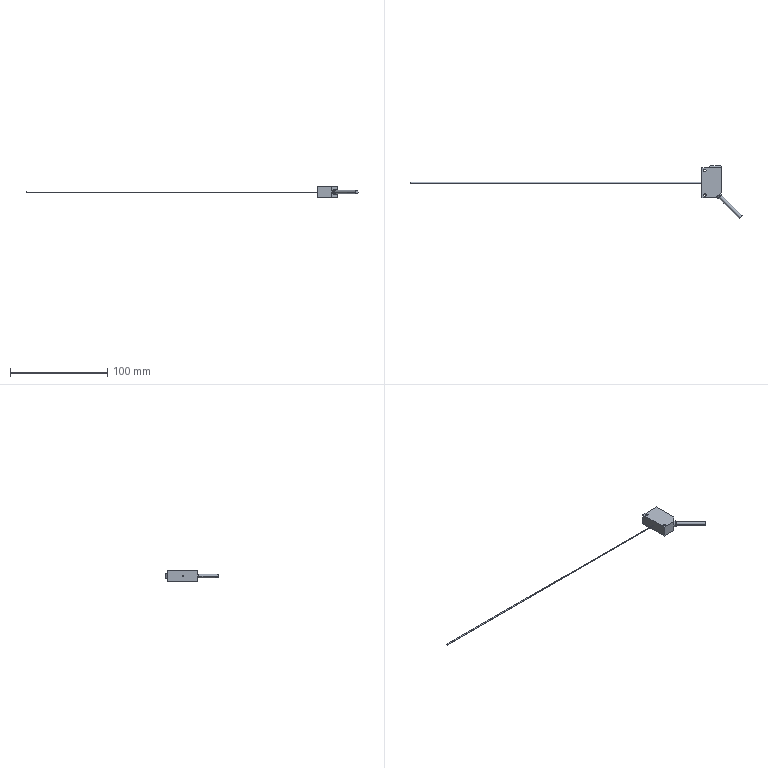Part | STEP file | Photoelectric sensor CX421 (NPN, 300mm) | 1 solid | 30 faces | box 341.148 x 54.448 x 11.2 mm | volume 7391 mm3 | cylinder 14 | plane 14 | cone 2 | commonest cylinder face diameters 2.5 x4 4 x4 1 x2 3.7 x2 6 x2